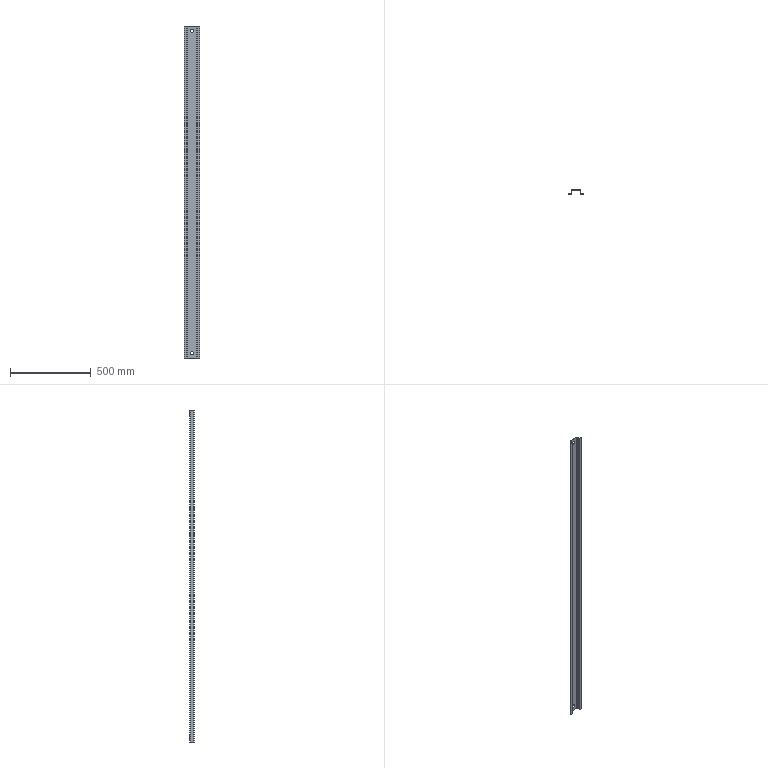Part | SolidWorks | features Cut 1, EdgeFlange 1, FlatPattern 1, ICE 1, SMBaseFlange 1, SheetMetal 1 | 1 solid | 42 faces | box 98.4 x 25 x 2051 mm | volume 236423 mm3 | plane 30 | cylinder 12 | commonest cylinder face diameters 2 x4 3.6 x4 20 x4
STEP:
#1=CARTESIAN_POINT('',(10.,-0.8,-995.5));
#2=VERTEX_POINT('',#1);
#3=CARTESIAN_POINT('',(-10.,-0.8,-995.5));
#4=VERTEX_POINT('',#3);
#5=CARTESIAN_POINT('',(0.,-0.8,-995.5));
#6=DIRECTION('',(0.,1.,0.));
#7=DIRECTION('',(-1.,0.,0.));
#8=AXIS2_PLACEMENT_3D('',#5,#6,#7);
#9=CIRCLE('',#8,10.);
#10=EDGE_CURVE('',#2,#4,#9,.T.);
#11=ORIENTED_EDGE('',*,*,#10,.F.);
#12=CARTESIAN_POINT('',(10.,0.,-995.5));
#13=VERTEX_POINT('',#12);
#14=CARTESIAN_POINT('',(10.,-10.,-995.5));
#15=DIRECTION('',(0.,1.,0.));
#16=VECTOR('',#15,1000.);
#17=LINE('',#14,#16);
#18=EDGE_CURVE('',#2,#13,#17,.T.);
#19=ORIENTED_EDGE('',*,*,#18,.T.);
#20=CARTESIAN_POINT('',(-10.,0.,-995.5));
#21=VERTEX_POINT('',#20);
#22=CARTESIAN_POINT('',(0.,0.,-995.5));
#23=DIRECTION('',(0.,1.,0.));
#24=DIRECTION('',(-1.,0.,0.));
#25=AXIS2_PLACEMENT_3D('',#22,#23,#24);
#26=CIRCLE('',#25,10.);
#27=EDGE_CURVE('',#13,#21,#26,.T.);
#28=ORIENTED_EDGE('',*,*,#27,.T.);
#29=CARTESIAN_POINT('',(-10.,-10.,-995.5));
#30=DIRECTION('',(0.,1.,0.));
#31=VECTOR('',#30,1000.);
#32=LINE('',#29,#31);
#33=EDGE_CURVE('',#4,#21,#32,.T.);
#34=ORIENTED_EDGE('',*,*,#33,.F.);
#35=EDGE_LOOP('',(#11,#19,#28,#34));
#36=FACE_OUTER_BOUND('',#35,.T.);
#37=CARTESIAN_POINT('',(0.,-10.,-995.5));
#38=DIRECTION('',(0.,1.,0.));
#39=DIRECTION('',(-1.,0.,0.));
#40=AXIS2_PLACEMENT_3D('',#37,#38,#39);
#41=CYLINDRICAL_SURFACE('',#40,10.);
#42=ADVANCED_FACE('',(#36),#41,.F.);
#43=CARTESIAN_POINT('',(10.,-0.8,995.5));
#44=VERTEX_POINT('',#43);
#45=CARTESIAN_POINT('',(-10.,-0.8,995.5));
#46=VERTEX_POINT('',#45);
#47=CARTESIAN_POINT('',(0.,-0.8,995.5));
#48=DIRECTION('',(0.,1.,0.));
#49=DIRECTION('',(-1.,0.,0.));
#50=AXIS2_PLACEMENT_3D('',#47,#48,#49);
#51=CIRCLE('',#50,10.);
#52=EDGE_CURVE('',#44,#46,#51,.T.);
#53=ORIENTED_EDGE('',*,*,#52,.F.);
#54=CARTESIAN_POINT('',(10.,0.,995.5));
#55=VERTEX_POINT('',#54);
#56=CARTESIAN_POINT('',(10.,-10.,995.5));
#57=DIRECTION('',(0.,1.,0.));
#58=VECTOR('',#57,1000.);
#59=LINE('',#56,#58);
#60=EDGE_CURVE('',#44,#55,#59,.T.);
#61=ORIENTED_EDGE('',*,*,#60,.T.);
#62=CARTESIAN_POINT('',(-10.,0.,995.5));
#63=VERTEX_POINT('',#62);
#64=CARTESIAN_POINT('',(0.,0.,995.5));
#65=DIRECTION('',(0.,1.,0.));
#66=DIRECTION('',(1.,0.,0.));
#67=AXIS2_PLACEMENT_3D('',#64,#65,#66);
#68=CIRCLE('',#67,10.);
#69=EDGE_CURVE('',#55,#63,#68,.T.);
#70=ORIENTED_EDGE('',*,*,#69,.T.);
#71=CARTESIAN_POINT('',(-10.,-10.,995.5));
#72=DIRECTION('',(0.,1.,0.));
#73=VECTOR('',#72,1000.);
#74=LINE('',#71,#73);
#75=EDGE_CURVE('',#46,#63,#74,.T.);
#76=ORIENTED_EDGE('',*,*,#75,.F.);
#77=EDGE_LOOP('',(#53,#61,#70,#76));
#78=FACE_OUTER_BOUND('',#77,.T.);
#79=CARTESIAN_POINT('',(0.,-10.,995.5));
#80=DIRECTION('',(0.,1.,0.));
#81=DIRECTION('',(-1.,0.,0.));
#82=AXIS2_PLACEMENT_3D('',#79,#80,#81);
#83=CYLINDRICAL_SURFACE('',#82,10.);
#84=ADVANCED_FACE('',(#78),#83,.F.);
#85=CARTESIAN_POINT('',(29.2,-23.2,-1025.5));
#86=VERTEX_POINT('',#85);
#87=CARTESIAN_POINT('',(29.2,-23.2,1025.5));
#88=VERTEX_POINT('',#87);
#89=CARTESIAN_POINT('',(29.2,-23.2,-1025.5));
#90=DIRECTION('',(0.,0.,1.));
#91=VECTOR('',#90,1000.);
#92=LINE('',#89,#91);
#93=EDGE_CURVE('',#86,#88,#92,.T.);
#94=ORIENTED_EDGE('',*,*,#93,.T.);
#95=CARTESIAN_POINT('',(29.2,-1.8,1025.5));
#96=VERTEX_POINT('',#95);
#97=CARTESIAN_POINT('',(29.2,0.,1025.5));
#98=DIRECTION('',(0.,-1.,0.));
#99=VECTOR('',#98,1000.);
#100=LINE('',#97,#99);
#101=EDGE_CURVE('',#96,#88,#100,.T.);
#102=ORIENTED_EDGE('',*,*,#101,.F.);
#103=CARTESIAN_POINT('',(29.2,-1.8,-1025.5));
#104=VERTEX_POINT('',#103);
#105=CARTESIAN_POINT('',(29.2,-1.8,1025.5));
#106=DIRECTION('',(0.,0.,-1.));
#107=VECTOR('',#106,1000.);
#108=LINE('',#105,#107);
#109=EDGE_CURVE('',#96,#104,#108,.T.);
#110=ORIENTED_EDGE('',*,*,#109,.T.);
#111=CARTESIAN_POINT('',(29.2,0.,-1025.5));
#112=DIRECTION('',(0.,-1.,0.));
#113=VECTOR('',#112,1000.);
#114=LINE('',#111,#113);
#115=EDGE_CURVE('',#104,#86,#114,.T.);
#116=ORIENTED_EDGE('',*,*,#115,.T.);
#117=EDGE_LOOP('',(#94,#102,#110,#116));
#118=FACE_OUTER_BOUND('',#117,.T.);
#119=CARTESIAN_POINT('',(29.2,0.,1025.5));
#120=DIRECTION('',(1.,0.,0.));
#121=DIRECTION('',(0.,1.,0.));
#122=AXIS2_PLACEMENT_3D('',#119,#120,#121);
#123=PLANE('',#122);
#124=ADVANCED_FACE('',(#118),#123,.F.);
#125=CARTESIAN_POINT('',(30.,-1.8,1025.5));
#126=VERTEX_POINT('',#125);
#127=CARTESIAN_POINT('',(30.,-23.2,1025.5));
#128=VERTEX_POINT('',#127);
#129=CARTESIAN_POINT('',(30.,0.,1025.5));
#130=DIRECTION('',(0.,-1.,0.));
#131=VECTOR('',#130,1000.);
#132=LINE('',#129,#131);
#133=EDGE_CURVE('',#126,#128,#132,.T.);
#134=ORIENTED_EDGE('',*,*,#133,.T.);
#135=CARTESIAN_POINT('',(30.,-23.2,-1025.5));
#136=VERTEX_POINT('',#135);
#137=CARTESIAN_POINT('',(30.,-23.2,-1025.5));
#138=DIRECTION('',(0.,0.,1.));
#139=VECTOR('',#138,1000.);
#140=LINE('',#137,#139);
#141=EDGE_CURVE('',#136,#128,#140,.T.);
#142=ORIENTED_EDGE('',*,*,#141,.F.);
#143=CARTESIAN_POINT('',(30.,-1.8,-1025.5));
#144=VERTEX_POINT('',#143);
#145=CARTESIAN_POINT('',(30.,0.,-1025.5));
#146=DIRECTION('',(0.,-1.,0.));
#147=VECTOR('',#146,1000.);
#148=LINE('',#145,#147);
#149=EDGE_CURVE('',#144,#136,#148,.T.);
#150=ORIENTED_EDGE('',*,*,#149,.F.);
#151=CARTESIAN_POINT('',(30.,-1.8,1025.5));
#152=DIRECTION('',(0.,0.,-1.));
#153=VECTOR('',#152,1000.);
#154=LINE('',#151,#153);
#155=EDGE_CURVE('',#126,#144,#154,.T.);
#156=ORIENTED_EDGE('',*,*,#155,.F.);
#157=EDGE_LOOP('',(#134,#142,#150,#156));
#158=FACE_OUTER_BOUND('',#157,.T.);
#159=CARTESIAN_POINT('',(30.,0.,1025.5));
#160=DIRECTION('',(1.,0.,0.));
#161=DIRECTION('',(0.,1.,0.));
#162=AXIS2_PLACEMENT_3D('',#159,#160,#161);
#163=PLANE('',#162);
#164=ADVANCED_FACE('',(#158),#163,.T.);
#165=CARTESIAN_POINT('',(30.,-23.2,-1025.5));
#166=DIRECTION('',(-1.,0.,0.));
#167=VECTOR('',#166,1000.);
#168=LINE('',#165,#167);
#169=EDGE_CURVE('',#136,#86,#168,.T.);
#170=ORIENTED_EDGE('',*,*,#169,.T.);
#171=ORIENTED_EDGE('',*,*,#115,.F.);
#172=CARTESIAN_POINT('',(29.2,-1.8,-1025.5));
#173=DIRECTION('',(1.,0.,0.));
#174=VECTOR('',#173,1000.);
#175=LINE('',#172,#174);
#176=EDGE_CURVE('',#104,#144,#175,.T.);
#177=ORIENTED_EDGE('',*,*,#176,.T.);
#178=ORIENTED_EDGE('',*,*,#149,.T.);
#179=EDGE_LOOP('',(#170,#171,#177,#178));
#180=FACE_OUTER_BOUND('',#179,.T.);
#181=CARTESIAN_POINT('',(28.2,-1.8,-1025.5));
#182=DIRECTION('',(0.,0.,1.));
#183=DIRECTION('',(1.,0.,0.));
#184=AXIS2_PLACEMENT_3D('',#181,#182,#183);
#185=PLANE('',#184);
#186=ADVANCED_FACE('',(#180),#185,.F.);
#187=CARTESIAN_POINT('',(-30.,-23.2,-1025.5));
#188=VERTEX_POINT('',#187);
#189=CARTESIAN_POINT('',(-30.,-1.8,-1025.5));
#190=VERTEX_POINT('',#189);
#191=CARTESIAN_POINT('',(-30.,-25.,-1025.5));
#192=DIRECTION('',(0.,1.,0.));
#193=VECTOR('',#192,1000.);
#194=LINE('',#191,#193);
#195=EDGE_CURVE('',#188,#190,#194,.T.);
#196=ORIENTED_EDGE('',*,*,#195,.F.);
#197=CARTESIAN_POINT('',(-30.,-23.2,1025.5));
#198=VERTEX_POINT('',#197);
#199=CARTESIAN_POINT('',(-30.,-23.2,1025.5));
#200=DIRECTION('',(0.,0.,-1.));
#201=VECTOR('',#200,1000.);
#202=LINE('',#199,#201);
#203=EDGE_CURVE('',#198,#188,#202,.T.);
#204=ORIENTED_EDGE('',*,*,#203,.F.);
#205=CARTESIAN_POINT('',(-30.,-1.8,1025.5));
#206=VERTEX_POINT('',#205);
#207=CARTESIAN_POINT('',(-30.,-25.,1025.5));
#208=DIRECTION('',(0.,1.,0.));
#209=VECTOR('',#208,1000.);
#210=LINE('',#207,#209);
#211=EDGE_CURVE('',#198,#206,#210,.T.);
#212=ORIENTED_EDGE('',*,*,#211,.T.);
#213=CARTESIAN_POINT('',(-30.,-1.8,1025.5));
#214=DIRECTION('',(0.,0.,-1.));
#215=VECTOR('',#214,1000.);
#216=LINE('',#213,#215);
#217=EDGE_CURVE('',#206,#190,#216,.T.);
#218=ORIENTED_EDGE('',*,*,#217,.T.);
#219=EDGE_LOOP('',(#196,#204,#212,#218));
#220=FACE_OUTER_BOUND('',#219,.T.);
#221=CARTESIAN_POINT('',(-30.,-25.,1025.5));
#222=DIRECTION('',(-1.,0.,0.));
#223=DIRECTION('',(0.,0.,1.));
#224=AXIS2_PLACEMENT_3D('',#221,#222,#223);
#225=PLANE('',#224);
#226=ADVANCED_FACE('',(#220),#225,.T.);
#227=CARTESIAN_POINT('',(-29.2,-23.2,1025.5));
#228=VERTEX_POINT('',#227);
#229=CARTESIAN_POINT('',(-29.2,-23.2,-1025.5));
#230=VERTEX_POINT('',#229);
#231=CARTESIAN_POINT('',(-29.2,-23.2,1025.5));
#232=DIRECTION('',(0.,0.,-1.));
#233=VECTOR('',#232,1000.);
#234=LINE('',#231,#233);
#235=EDGE_CURVE('',#228,#230,#234,.T.);
#236=ORIENTED_EDGE('',*,*,#235,.T.);
#237=CARTESIAN_POINT('',(-29.2,-1.8,-1025.5));
#238=VERTEX_POINT('',#237);
#239=CARTESIAN_POINT('',(-29.2,-25.,-1025.5));
#240=DIRECTION('',(0.,1.,0.));
#241=VECTOR('',#240,1000.);
#242=LINE('',#239,#241);
#243=EDGE_CURVE('',#230,#238,#242,.T.);
#244=ORIENTED_EDGE('',*,*,#243,.T.);
#245=CARTESIAN_POINT('',(-29.2,-1.8,1025.5));
#246=VERTEX_POINT('',#245);
#247=CARTESIAN_POINT('',(-29.2,-1.8,1025.5));
#248=DIRECTION('',(0.,0.,-1.));
#249=VECTOR('',#248,1000.);
#250=LINE('',#247,#249);
#251=EDGE_CURVE('',#246,#238,#250,.T.);
#252=ORIENTED_EDGE('',*,*,#251,.F.);
#253=CARTESIAN_POINT('',(-29.2,-25.,1025.5));
#254=DIRECTION('',(0.,1.,0.));
#255=VECTOR('',#254,1000.);
#256=LINE('',#253,#255);
#257=EDGE_CURVE('',#228,#246,#256,.T.);
#258=ORIENTED_EDGE('',*,*,#257,.F.);
#259=EDGE_LOOP('',(#236,#244,#252,#258));
#260=FACE_OUTER_BOUND('',#259,.T.);
#261=CARTESIAN_POINT('',(-29.2,-25.,1025.5));
#262=DIRECTION('',(-1.,0.,0.));
#263=DIRECTION('',(0.,0.,1.));
#264=AXIS2_PLACEMENT_3D('',#261,#262,#263);
#265=PLANE('',#264);
#266=ADVANCED_FACE('',(#260),#265,.F.);
#267=ORIENTED_EDGE('',*,*,#211,.F.);
#268=CARTESIAN_POINT('',(-30.,-23.2,1025.5));
#269=DIRECTION('',(1.,0.,0.));
#270=VECTOR('',#269,1000.);
#271=LINE('',#268,#270);
#272=EDGE_CURVE('',#198,#228,#271,.T.);
#273=ORIENTED_EDGE('',*,*,#272,.T.);
#274=ORIENTED_EDGE('',*,*,#257,.T.);
#275=CARTESIAN_POINT('',(-29.2,-1.8,1025.5));
#276=DIRECTION('',(-1.,0.,0.));
#277=VECTOR('',#276,1000.);
#278=LINE('',#275,#277);
#279=EDGE_CURVE('',#246,#206,#278,.T.);
#280=ORIENTED_EDGE('',*,*,#279,.T.);
#281=EDGE_LOOP('',(#267,#273,#274,#280));
#282=FACE_OUTER_BOUND('',#281,.T.);
#283=CARTESIAN_POINT('',(28.2,-1.8,1025.5));
#284=DIRECTION('',(0.,0.,1.));
#285=DIRECTION('',(1.,0.,0.));
#286=AXIS2_PLACEMENT_3D('',#283,#284,#285);
#287=PLANE('',#286);
#288=ADVANCED_FACE('',(#282),#287,.T.);
#289=CARTESIAN_POINT('',(-28.2,0.,1025.5));
#290=VERTEX_POINT('',#289);
#291=CARTESIAN_POINT('',(-28.2,-0.8,1025.5));
#292=VERTEX_POINT('',#291);
#293=CARTESIAN_POINT('',(-28.2,0.,1025.5));
#294=DIRECTION('',(0.,-1.,0.));
#295=VECTOR('',#294,1000.);
#296=LINE('',#293,#295);
#297=EDGE_CURVE('',#290,#292,#296,.T.);
#298=ORIENTED_EDGE('',*,*,#297,.F.);
#299=CARTESIAN_POINT('',(-28.2,-1.8,1025.5));
#300=DIRECTION('',(0.,0.,-1.));
#301=DIRECTION('',(1.,0.,0.));
#302=AXIS2_PLACEMENT_3D('',#299,#300,#301);
#303=CIRCLE('',#302,1.8);
#304=EDGE_CURVE('',#206,#290,#303,.T.);
#305=ORIENTED_EDGE('',*,*,#304,.F.);
#306=ORIENTED_EDGE('',*,*,#279,.F.);
#307=CARTESIAN_POINT('',(-28.2,-1.8,1025.5));
#308=DIRECTION('',(0.,0.,-1.));
#309=DIRECTION('',(1.,0.,0.));
#310=AXIS2_PLACEMENT_3D('',#307,#308,#309);
#311=CIRCLE('',#310,1.);
#312=EDGE_CURVE('',#246,#292,#311,.T.);
#313=ORIENTED_EDGE('',*,*,#312,.T.);
#314=EDGE_LOOP('',(#298,#305,#306,#313));
#315=FACE_OUTER_BOUND('',#314,.T.);
#316=CARTESIAN_POINT('',(-28.2,0.,1025.5));
#317=DIRECTION('',(0.,0.,1.));
#318=DIRECTION('',(1.,0.,0.));
#319=AXIS2_PLACEMENT_3D('',#316,#317,#318);
#320=PLANE('',#319);
#321=ADVANCED_FACE('',(#315),#320,.T.);
#322=CARTESIAN_POINT('',(28.2,0.,1025.5));
#323=VERTEX_POINT('',#322);
#324=CARTESIAN_POINT('',(-30.,0.,1025.5));
#325=DIRECTION('',(1.,0.,0.));
#326=VECTOR('',#325,1000.);
#327=LINE('',#324,#326);
#328=EDGE_CURVE('',#290,#323,#327,.T.);
#329=ORIENTED_EDGE('',*,*,#328,.F.);
#330=ORIENTED_EDGE('',*,*,#297,.T.);
#331=CARTESIAN_POINT('',(28.2,-0.8,1025.5));
#332=VERTEX_POINT('',#331);
#333=CARTESIAN_POINT('',(-30.,-0.8,1025.5));
#334=DIRECTION('',(1.,0.,0.));
#335=VECTOR('',#334,1000.);
#336=LINE('',#333,#335);
#337=EDGE_CURVE('',#292,#332,#336,.T.);
#338=ORIENTED_EDGE('',*,*,#337,.T.);
#339=CARTESIAN_POINT('',(28.2,-0.8,1025.5));
#340=DIRECTION('',(0.,1.,0.));
#341=VECTOR('',#340,1000.);
#342=LINE('',#339,#341);
#343=EDGE_CURVE('',#332,#323,#342,.T.);
#344=ORIENTED_EDGE('',*,*,#343,.T.);
#345=EDGE_LOOP('',(#329,#330,#338,#344));
#346=FACE_OUTER_BOUND('',#345,.T.);
#347=CARTESIAN_POINT('',(-29.2,-1.8,1025.5));
#348=DIRECTION('',(0.,0.,1.));
#349=DIRECTION('',(1.,0.,0.));
#350=AXIS2_PLACEMENT_3D('',#347,#348,#349);
#351=PLANE('',#350);
#352=ADVANCED_FACE('',(#346),#351,.T.);
#353=CARTESIAN_POINT('',(-30.,-1.8,-1025.5));
#354=DIRECTION('',(1.,0.,0.));
#355=VECTOR('',#354,1000.);
#356=LINE('',#353,#355);
#357=EDGE_CURVE('',#190,#238,#356,.T.);
#358=ORIENTED_EDGE('',*,*,#357,.F.);
#359=CARTESIAN_POINT('',(-28.2,0.,-1025.5));
#360=VERTEX_POINT('',#359);
#361=CARTESIAN_POINT('',(-28.2,-1.8,-1025.5));
#362=DIRECTION('',(0.,0.,-1.));
#363=DIRECTION('',(1.,0.,0.));
#364=AXIS2_PLACEMENT_3D('',#361,#362,#363);
#365=CIRCLE('',#364,1.8);
#366=EDGE_CURVE('',#190,#360,#365,.T.);
#367=ORIENTED_EDGE('',*,*,#366,.T.);
#368=CARTESIAN_POINT('',(-28.2,-0.8,-1025.5));
#369=VERTEX_POINT('',#368);
#370=CARTESIAN_POINT('',(-28.2,-0.8,-1025.5));
#371=DIRECTION('',(0.,1.,0.));
#372=VECTOR('',#371,1000.);
#373=LINE('',#370,#372);
#374=EDGE_CURVE('',#369,#360,#373,.T.);
#375=ORIENTED_EDGE('',*,*,#374,.F.);
#376=CARTESIAN_POINT('',(-28.2,-1.8,-1025.5));
#377=DIRECTION('',(0.,0.,-1.));
#378=DIRECTION('',(1.,0.,0.));
#379=AXIS2_PLACEMENT_3D('',#376,#377,#378);
#380=CIRCLE('',#379,1.);
#381=EDGE_CURVE('',#238,#369,#380,.T.);
#382=ORIENTED_EDGE('',*,*,#381,.F.);
#383=EDGE_LOOP('',(#358,#367,#375,#382));
#384=FACE_OUTER_BOUND('',#383,.T.);
#385=CARTESIAN_POINT('',(-30.,-1.8,-1025.5));
#386=DIRECTION('',(0.,0.,-1.));
#387=DIRECTION('',(-1.,0.,0.));
#388=AXIS2_PLACEMENT_3D('',#385,#386,#387);
#389=PLANE('',#388);
#390=ADVANCED_FACE('',(#384),#389,.T.);
#391=CARTESIAN_POINT('',(-30.,-23.2,-1025.5));
#392=DIRECTION('',(1.,0.,0.));
#393=VECTOR('',#392,1000.);
#394=LINE('',#391,#393);
#395=EDGE_CURVE('',#188,#230,#394,.T.);
#396=ORIENTED_EDGE('',*,*,#395,.F.);
#397=ORIENTED_EDGE('',*,*,#195,.T.);
#398=ORIENTED_EDGE('',*,*,#357,.T.);
#399=ORIENTED_EDGE('',*,*,#243,.F.);
#400=EDGE_LOOP('',(#396,#397,#398,#399));
#401=FACE_OUTER_BOUND('',#400,.T.);
#402=CARTESIAN_POINT('',(-28.2,-0.8,-1025.5));
#403=DIRECTION('',(0.,0.,-1.));
#404=DIRECTION('',(-1.,0.,0.));
#405=AXIS2_PLACEMENT_3D('',#402,#403,#404);
#406=PLANE('',#405);
#407=ADVANCED_FACE('',(#401),#406,.T.);
#408=CARTESIAN_POINT('',(30.,-1.8,1025.5));
#409=DIRECTION('',(-1.,0.,0.));
#410=VECTOR('',#409,1000.);
#411=LINE('',#408,#410);
#412=EDGE_CURVE('',#126,#96,#411,.T.);
#413=ORIENTED_EDGE('',*,*,#412,.F.);
#414=CARTESIAN_POINT('',(28.2,-1.8,1025.5));
#415=DIRECTION('',(0.,0.,-1.));
#416=DIRECTION('',(1.,0.,0.));
#417=AXIS2_PLACEMENT_3D('',#414,#415,#416);
#418=CIRCLE('',#417,1.8);
#419=EDGE_CURVE('',#323,#126,#418,.T.);
#420=ORIENTED_EDGE('',*,*,#419,.F.);
#421=ORIENTED_EDGE('',*,*,#343,.F.);
#422=CARTESIAN_POINT('',(28.2,-1.8,1025.5));
#423=DIRECTION('',(0.,0.,-1.));
#424=DIRECTION('',(1.,0.,0.));
#425=AXIS2_PLACEMENT_3D('',#422,#423,#424);
#426=CIRCLE('',#425,1.);
#427=EDGE_CURVE('',#332,#96,#426,.T.);
#428=ORIENTED_EDGE('',*,*,#427,.T.);
#429=EDGE_LOOP('',(#413,#420,#421,#428));
#430=FACE_OUTER_BOUND('',#429,.T.);
#431=CARTESIAN_POINT('',(30.,-1.8,1025.5));
#432=DIRECTION('',(0.,0.,1.));
#433=DIRECTION('',(1.,0.,0.));
#434=AXIS2_PLACEMENT_3D('',#431,#432,#433);
#435=PLANE('',#434);
#436=ADVANCED_FACE('',(#430),#435,.T.);
#437=CARTESIAN_POINT('',(30.,-23.2,1025.5));
#438=DIRECTION('',(-1.,0.,0.));
#439=VECTOR('',#438,1000.);
#440=LINE('',#437,#439);
#441=EDGE_CURVE('',#128,#88,#440,.T.);
#442=ORIENTED_EDGE('',*,*,#441,.F.);
#443=ORIENTED_EDGE('',*,*,#133,.F.);
#444=ORIENTED_EDGE('',*,*,#412,.T.);
#445=ORIENTED_EDGE('',*,*,#101,.T.);
#446=EDGE_LOOP('',(#442,#443,#444,#445));
#447=FACE_OUTER_BOUND('',#446,.T.);
#448=CARTESIAN_POINT('',(28.2,-0.8,1025.5));
#449=DIRECTION('',(0.,0.,1.));
#450=DIRECTION('',(1.,0.,0.));
#451=AXIS2_PLACEMENT_3D('',#448,#449,#450);
#452=PLANE('',#451);
#453=ADVANCED_FACE('',(#447),#452,.T.);
#454=CARTESIAN_POINT('',(28.2,0.,-1025.5));
#455=VERTEX_POINT('',#454);
#456=CARTESIAN_POINT('',(28.2,-0.8,-1025.5));
#457=VERTEX_POINT('',#456);
#458=CARTESIAN_POINT('',(28.2,0.,-1025.5));
#459=DIRECTION('',(0.,-1.,0.));
#460=VECTOR('',#459,1000.);
#461=LINE('',#458,#460);
#462=EDGE_CURVE('',#455,#457,#461,.T.);
#463=ORIENTED_EDGE('',*,*,#462,.F.);
#464=CARTESIAN_POINT('',(28.2,-1.8,-1025.5));
#465=DIRECTION('',(0.,0.,-1.));
#466=DIRECTION('',(1.,0.,0.));
#467=AXIS2_PLACEMENT_3D('',#464,#465,#466);
#468=CIRCLE('',#467,1.8);
#469=EDGE_CURVE('',#455,#144,#468,.T.);
#470=ORIENTED_EDGE('',*,*,#469,.T.);
#471=ORIENTED_EDGE('',*,*,#176,.F.);
#472=CARTESIAN_POINT('',(28.2,-1.8,-1025.5));
#473=DIRECTION('',(0.,0.,-1.));
#474=DIRECTION('',(1.,0.,0.));
#475=AXIS2_PLACEMENT_3D('',#472,#473,#474);
#476=CIRCLE('',#475,1.);
#477=EDGE_CURVE('',#457,#104,#476,.T.);
#478=ORIENTED_EDGE('',*,*,#477,.F.);
#479=EDGE_LOOP('',(#463,#470,#471,#478));
#480=FACE_OUTER_BOUND('',#479,.T.);
#481=CARTESIAN_POINT('',(28.2,0.,-1025.5));
#482=DIRECTION('',(0.,0.,-1.));
#483=DIRECTION('',(-1.,0.,0.));
#484=AXIS2_PLACEMENT_3D('',#481,#482,#483);
#485=PLANE('',#484);
#486=ADVANCED_FACE('',(#480),#485,.T.);
#487=CARTESIAN_POINT('',(-30.,0.,-1025.5));
#488=DIRECTION('',(1.,0.,0.));
#489=VECTOR('',#488,1000.);
#490=LINE('',#487,#489);
#491=EDGE_CURVE('',#360,#455,#490,.T.);
#492=ORIENTED_EDGE('',*,*,#491,.T.);
#493=ORIENTED_EDGE('',*,*,#462,.T.);
#494=CARTESIAN_POINT('',(-30.,-0.8,-1025.5));
#495=DIRECTION('',(1.,0.,0.));
#496=VECTOR('',#495,1000.);
#497=LINE('',#494,#496);
#498=EDGE_CURVE('',#369,#457,#497,.T.);
#499=ORIENTED_EDGE('',*,*,#498,.F.);
#500=ORIENTED_EDGE('',*,*,#374,.T.);
#501=EDGE_LOOP('',(#492,#493,#499,#500));
#502=FACE_OUTER_BOUND('',#501,.T.);
#503=CARTESIAN_POINT('',(29.2,-1.8,-1025.5));
#504=DIRECTION('',(0.,0.,-1.));
#505=DIRECTION('',(-1.,0.,0.));
#506=AXIS2_PLACEMENT_3D('',#503,#504,#505);
#507=PLANE('',#506);
#508=ADVANCED_FACE('',(#502),#507,.T.);
#509=ORIENTED_EDGE('',*,*,#469,.F.);
#510=CARTESIAN_POINT('',(28.2,0.,1025.5));
#511=DIRECTION('',(0.,0.,-1.));
#512=VECTOR('',#511,1000.);
#513=LINE('',#510,#512);
#514=EDGE_CURVE('',#323,#455,#513,.T.);
#515=ORIENTED_EDGE('',*,*,#514,.F.);
#516=ORIENTED_EDGE('',*,*,#419,.T.);
#517=ORIENTED_EDGE('',*,*,#155,.T.);
#518=EDGE_LOOP('',(#509,#515,#516,#517));
#519=FACE_OUTER_BOUND('',#518,.T.);
#520=CARTESIAN_POINT('',(28.2,-1.8,1025.5));
#521=DIRECTION('',(0.,0.,-1.));
#522=DIRECTION('',(-1.,0.,0.));
#523=AXIS2_PLACEMENT_3D('',#520,#521,#522);
#524=CYLINDRICAL_SURFACE('',#523,1.8);
#525=ADVANCED_FACE('',(#519),#524,.T.);
#526=CARTESIAN_POINT('',(0.,0.,-995.5));
#527=DIRECTION('',(0.,1.,0.));
#528=DIRECTION('',(-1.,0.,0.));
#529=AXIS2_PLACEMENT_3D('',#526,#527,#528);
#530=CIRCLE('',#529,10.);
#531=EDGE_CURVE('',#21,#13,#530,.T.);
#532=ORIENTED_EDGE('',*,*,#531,.F.);
#533=ORIENTED_EDGE('',*,*,#27,.F.);
#534=EDGE_LOOP('',(#532,#533));
#535=FACE_BOUND('',#534,.T.);
#536=CARTESIAN_POINT('',(0.,0.,995.5));
#537=DIRECTION('',(0.,1.,0.));
#538=DIRECTION('',(1.,0.,0.));
#539=AXIS2_PLACEMENT_3D('',#536,#537,#538);
#540=CIRCLE('',#539,10.);
#541=EDGE_CURVE('',#63,#55,#540,.T.);
#542=ORIENTED_EDGE('',*,*,#541,.F.);
#543=ORIENTED_EDGE('',*,*,#69,.F.);
#544=EDGE_LOOP('',(#542,#543));
#545=FACE_BOUND('',#544,.T.);
#546=ORIENTED_EDGE('',*,*,#491,.F.);
#547=CARTESIAN_POINT('',(-28.2,0.,1025.5));
#548=DIRECTION('',(0.,0.,-1.));
#549=VECTOR('',#548,1000.);
#550=LINE('',#547,#549);
#551=EDGE_CURVE('',#290,#360,#550,.T.);
#552=ORIENTED_EDGE('',*,*,#551,.F.);
#553=ORIENTED_EDGE('',*,*,#328,.T.);
#554=ORIENTED_EDGE('',*,*,#514,.T.);
#555=EDGE_LOOP('',(#546,#552,#553,#554));
#556=FACE_OUTER_BOUND('',#555,.T.);
#557=CARTESIAN_POINT('',(-30.,0.,1025.5));
#558=DIRECTION('',(0.,1.,0.));
#559=DIRECTION('',(-1.,0.,0.));
#560=AXIS2_PLACEMENT_3D('',#557,#558,#559);
#561=PLANE('',#560);
#562=ADVANCED_FACE('',(#535,#545,#556),#561,.T.);
#563=ORIENTED_EDGE('',*,*,#366,.F.);
#564=ORIENTED_EDGE('',*,*,#217,.F.);
#565=ORIENTED_EDGE('',*,*,#304,.T.);
#566=ORIENTED_EDGE('',*,*,#551,.T.);
#567=EDGE_LOOP('',(#563,#564,#565,#566));
#568=FACE_OUTER_BOUND('',#567,.T.);
#569=CARTESIAN_POINT('',(-28.2,-1.8,1025.5));
#570=DIRECTION('',(0.,0.,-1.));
#571=DIRECTION('',(-1.,0.,0.));
#572=AXIS2_PLACEMENT_3D('',#569,#570,#571);
#573=CYLINDRICAL_SURFACE('',#572,1.8);
#574=ADVANCED_FACE('',(#568),#573,.T.);
#575=ORIENTED_EDGE('',*,*,#381,.T.);
#576=CARTESIAN_POINT('',(-28.2,-0.8,1025.5));
#577=DIRECTION('',(0.,0.,-1.));
#578=VECTOR('',#577,1000.);
#579=LINE('',#576,#578);
#580=EDGE_CURVE('',#292,#369,#579,.T.);
#581=ORIENTED_EDGE('',*,*,#580,.F.);
#582=ORIENTED_EDGE('',*,*,#312,.F.);
#583=ORIENTED_EDGE('',*,*,#251,.T.);
#584=EDGE_LOOP('',(#575,#581,#582,#583));
#585=FACE_OUTER_BOUND('',#584,.T.);
#586=CARTESIAN_POINT('',(-28.2,-1.8,1025.5));
#587=DIRECTION('',(0.,0.,-1.));
#588=DIRECTION('',(-1.,0.,0.));
#589=AXIS2_PLACEMENT_3D('',#586,#587,#588);
#590=CYLINDRICAL_SURFACE('',#589,1.);
#591=ADVANCED_FACE('',(#585),#590,.F.);
#592=CARTESIAN_POINT('',(0.,-0.8,-995.5));
#593=DIRECTION('',(0.,1.,0.));
#594=DIRECTION('',(-1.,0.,0.));
#595=AXIS2_PLACEMENT_3D('',#592,#593,#594);
#596=CIRCLE('',#595,10.);
#597=EDGE_CURVE('',#4,#2,#596,.T.);
#598=ORIENTED_EDGE('',*,*,#597,.T.);
#599=ORIENTED_EDGE('',*,*,#10,.T.);
#600=EDGE_LOOP('',(#598,#599));
#601=FACE_BOUND('',#600,.T.);
#602=CARTESIAN_POINT('',(0.,-0.8,995.5));
#603=DIRECTION('',(0.,1.,0.));
#604=DIRECTION('',(-1.,0.,0.));
#605=AXIS2_PLACEMENT_3D('',#602,#603,#604);
#606=CIRCLE('',#605,10.);
#607=EDGE_CURVE('',#46,#44,#606,.T.);
#608=ORIENTED_EDGE('',*,*,#607,.T.);
#609=ORIENTED_EDGE('',*,*,#52,.T.);
#610=EDGE_LOOP('',(#608,#609));
#611=FACE_BOUND('',#610,.T.);
#612=ORIENTED_EDGE('',*,*,#498,.T.);
#613=CARTESIAN_POINT('',(28.2,-0.8,1025.5));
#614=DIRECTION('',(0.,0.,-1.));
#615=VECTOR('',#614,1000.);
#616=LINE('',#613,#615);
#617=EDGE_CURVE('',#332,#457,#616,.T.);
#618=ORIENTED_EDGE('',*,*,#617,.F.);
#619=ORIENTED_EDGE('',*,*,#337,.F.);
#620=ORIENTED_EDGE('',*,*,#580,.T.);
#621=EDGE_LOOP('',(#612,#618,#619,#620));
#622=FACE_OUTER_BOUND('',#621,.T.);
#623=CARTESIAN_POINT('',(-30.,-0.8,1025.5));
#624=DIRECTION('',(0.,1.,0.));
#625=DIRECTION('',(-1.,0.,0.));
#626=AXIS2_PLACEMENT_3D('',#623,#624,#625);
#627=PLANE('',#626);
#628=ADVANCED_FACE('',(#601,#611,#622),#627,.F.);
#629=ORIENTED_EDGE('',*,*,#477,.T.);
#630=ORIENTED_EDGE('',*,*,#109,.F.);
#631=ORIENTED_EDGE('',*,*,#427,.F.);
#632=ORIENTED_EDGE('',*,*,#617,.T.);
#633=EDGE_LOOP('',(#629,#630,#631,#632));
#634=FACE_OUTER_BOUND('',#633,.T.);
#635=CARTESIAN_POINT('',(28.2,-1.8,1025.5));
#636=DIRECTION('',(0.,0.,-1.));
#637=DIRECTION('',(-1.,0.,0.));
#638=AXIS2_PLACEMENT_3D('',#635,#636,#637);
#639=CYLINDRICAL_SURFACE('',#638,1.);
#640=ADVANCED_FACE('',(#634),#639,.F.);
#641=CARTESIAN_POINT('',(-31.,-24.2,-1025.5));
#642=VERTEX_POINT('',#641);
#643=CARTESIAN_POINT('',(-31.,-25.,-1025.5));
#644=VERTEX_POINT('',#643);
#645=CARTESIAN_POINT('',(-31.,-25.,-1025.5));
#646=DIRECTION('',(0.,-1.,0.));
#647=VECTOR('',#646,1000.);
#648=LINE('',#645,#647);
#649=EDGE_CURVE('',#642,#644,#648,.T.);
#650=ORIENTED_EDGE('',*,*,#649,.F.);
#651=CARTESIAN_POINT('',(-31.,-23.2,-1025.5));
#652=DIRECTION('',(0.,0.,-1.));
#653=DIRECTION('',(1.,0.,0.));
#654=AXIS2_PLACEMENT_3D('',#651,#652,#653);
#655=CIRCLE('',#654,1.);
#656=EDGE_CURVE('',#188,#642,#655,.T.);
#657=ORIENTED_EDGE('',*,*,#656,.F.);
#658=ORIENTED_EDGE('',*,*,#395,.T.);
#659=CARTESIAN_POINT('',(-31.,-23.2,-1025.5));
#660=DIRECTION('',(0.,0.,-1.));
#661=DIRECTION('',(1.,0.,0.));
#662=AXIS2_PLACEMENT_3D('',#659,#660,#661);
#663=CIRCLE('',#662,1.8);
#664=EDGE_CURVE('',#230,#644,#663,.T.);
#665=ORIENTED_EDGE('',*,*,#664,.T.);
#666=EDGE_LOOP('',(#650,#657,#658,#665));
#667=FACE_OUTER_BOUND('',#666,.T.);
#668=CARTESIAN_POINT('',(-31.,-23.2,-1025.5));
#669=DIRECTION('',(0.,0.,-1.));
#670=DIRECTION('',(-1.,0.,0.));
#671=AXIS2_PLACEMENT_3D('',#668,#669,#670);
#672=PLANE('',#671);
#673=ADVANCED_FACE('',(#667),#672,.T.);
#674=CARTESIAN_POINT('',(-31.,-24.2,1025.5));
#675=VERTEX_POINT('',#674);
#676=CARTESIAN_POINT('',(-31.,-23.2,1025.5));
#677=DIRECTION('',(0.,0.,1.));
#678=DIRECTION('',(1.,0.,0.));
#679=AXIS2_PLACEMENT_3D('',#676,#677,#678);
#680=CIRCLE('',#679,1.);
#681=EDGE_CURVE('',#675,#198,#680,.T.);
#682=ORIENTED_EDGE('',*,*,#681,.F.);
#683=CARTESIAN_POINT('',(-31.,-25.,1025.5));
#684=VERTEX_POINT('',#683);
#685=CARTESIAN_POINT('',(-31.,-24.2,1025.5));
#686=DIRECTION('',(0.,-1.,0.));
#687=VECTOR('',#686,1000.);
#688=LINE('',#685,#687);
#689=EDGE_CURVE('',#675,#684,#688,.T.);
#690=ORIENTED_EDGE('',*,*,#689,.T.);
#691=CARTESIAN_POINT('',(-31.,-23.2,1025.5));
#692=DIRECTION('',(0.,0.,1.));
#693=DIRECTION('',(1.,0.,0.));
#694=AXIS2_PLACEMENT_3D('',#691,#692,#693);
#695=CIRCLE('',#694,1.8);
#696=EDGE_CURVE('',#684,#228,#695,.T.);
#697=ORIENTED_EDGE('',*,*,#696,.T.);
#698=ORIENTED_EDGE('',*,*,#272,.F.);
#699=EDGE_LOOP('',(#682,#690,#697,#698));
#700=FACE_OUTER_BOUND('',#699,.T.);
#701=CARTESIAN_POINT('',(-31.,-23.2,1025.5));
#702=DIRECTION('',(0.,0.,-1.));
#703=DIRECTION('',(-1.,0.,0.));
#704=AXIS2_PLACEMENT_3D('',#701,#702,#703);
#705=PLANE('',#704);
#706=ADVANCED_FACE('',(#700),#705,.F.);
#707=ORIENTED_EDGE('',*,*,#235,.F.);
#708=ORIENTED_EDGE('',*,*,#696,.F.);
#709=CARTESIAN_POINT('',(-31.,-25.,-1025.5));
#710=DIRECTION('',(0.,0.,-1.));
#711=VECTOR('',#710,1000.);
#712=LINE('',#709,#711);
#713=EDGE_CURVE('',#684,#644,#712,.T.);
#714=ORIENTED_EDGE('',*,*,#713,.T.);
#715=ORIENTED_EDGE('',*,*,#664,.F.);
#716=EDGE_LOOP('',(#707,#708,#714,#715));
#717=FACE_OUTER_BOUND('',#716,.T.);
#718=CARTESIAN_POINT('',(-31.,-23.2,1025.5));
#719=DIRECTION('',(0.,0.,1.));
#720=DIRECTION('',(0.,-1.,0.));
#721=AXIS2_PLACEMENT_3D('',#718,#719,#720);
#722=CYLINDRICAL_SURFACE('',#721,1.8);
#723=ADVANCED_FACE('',(#717),#722,.T.);
#724=ORIENTED_EDGE('',*,*,#203,.T.);
#725=ORIENTED_EDGE('',*,*,#656,.T.);
#726=CARTESIAN_POINT('',(-31.,-24.2,-1025.5));
#727=DIRECTION('',(0.,0.,1.));
#728=VECTOR('',#727,1000.);
#729=LINE('',#726,#728);
#730=EDGE_CURVE('',#642,#675,#729,.T.);
#731=ORIENTED_EDGE('',*,*,#730,.T.);
#732=ORIENTED_EDGE('',*,*,#681,.T.);
#733=EDGE_LOOP('',(#724,#725,#731,#732));
#734=FACE_OUTER_BOUND('',#733,.T.);
#735=CARTESIAN_POINT('',(-31.,-23.2,1025.5));
#736=DIRECTION('',(0.,0.,1.));
#737=DIRECTION('',(0.,-1.,0.));
#738=AXIS2_PLACEMENT_3D('',#735,#736,#737);
#739=CYLINDRICAL_SURFACE('',#738,1.);
#740=ADVANCED_FACE('',(#734),#739,.F.);
#741=ORIENTED_EDGE('',*,*,#689,.F.);
#742=CARTESIAN_POINT('',(-49.2,-24.2,1025.5));
#743=VERTEX_POINT('',#742);
#744=CARTESIAN_POINT('',(-49.2,-24.2,1025.5));
#745=DIRECTION('',(-1.,0.,0.));
#746=VECTOR('',#745,1000.);
#747=LINE('',#744,#746);
#748=EDGE_CURVE('',#675,#743,#747,.T.);
#749=ORIENTED_EDGE('',*,*,#748,.T.);
#750=CARTESIAN_POINT('',(-49.2,-25.,1025.5));
#751=VERTEX_POINT('',#750);
#752=CARTESIAN_POINT('',(-49.2,-25.,1025.5));
#753=DIRECTION('',(0.,1.,0.));
#754=VECTOR('',#753,1000.);
#755=LINE('',#752,#754);
#756=EDGE_CURVE('',#751,#743,#755,.T.);
#757=ORIENTED_EDGE('',*,*,#756,.F.);
#758=CARTESIAN_POINT('',(0.,-25.,1025.5));
#759=DIRECTION('',(-1.,0.,0.));
#760=VECTOR('',#759,1000.);
#761=LINE('',#758,#760);
#762=EDGE_CURVE('',#684,#751,#761,.T.);
#763=ORIENTED_EDGE('',*,*,#762,.F.);
#764=EDGE_LOOP('',(#741,#749,#757,#763));
#765=FACE_OUTER_BOUND('',#764,.T.);
#766=CARTESIAN_POINT('',(-49.2,-25.,1025.5));
#767=DIRECTION('',(0.,0.,-1.));
#768=DIRECTION('',(-1.,0.,0.));
#769=AXIS2_PLACEMENT_3D('',#766,#767,#768);
#770=PLANE('',#769);
#771=ADVANCED_FACE('',(#765),#770,.F.);
#772=ORIENTED_EDGE('',*,*,#649,.T.);
#773=CARTESIAN_POINT('',(-49.2,-25.,-1025.5));
#774=VERTEX_POINT('',#773);
#775=CARTESIAN_POINT('',(0.,-25.,-1025.5));
#776=DIRECTION('',(1.,0.,0.));
#777=VECTOR('',#776,1000.);
#778=LINE('',#775,#777);
#779=EDGE_CURVE('',#774,#644,#778,.T.);
#780=ORIENTED_EDGE('',*,*,#779,.F.);
#781=CARTESIAN_POINT('',(-49.2,-24.2,-1025.5));
#782=VERTEX_POINT('',#781);
#783=CARTESIAN_POINT('',(-49.2,-25.,-1025.5));
#784=DIRECTION('',(0.,1.,0.));
#785=VECTOR('',#784,1000.);
#786=LINE('',#783,#785);
#787=EDGE_CURVE('',#774,#782,#786,.T.);
#788=ORIENTED_EDGE('',*,*,#787,.T.);
#789=CARTESIAN_POINT('',(-30.,-24.2,-1025.5));
#790=DIRECTION('',(1.,0.,0.));
#791=VECTOR('',#790,1000.);
#792=LINE('',#789,#791);
#793=EDGE_CURVE('',#782,#642,#792,.T.);
#794=ORIENTED_EDGE('',*,*,#793,.T.);
#795=EDGE_LOOP('',(#772,#780,#788,#794));
#796=FACE_OUTER_BOUND('',#795,.T.);
#797=CARTESIAN_POINT('',(-30.,-25.,-1025.5));
#798=DIRECTION('',(0.,0.,1.));
#799=DIRECTION('',(1.,0.,0.));
#800=AXIS2_PLACEMENT_3D('',#797,#798,#799);
#801=PLANE('',#800);
#802=ADVANCED_FACE('',(#796),#801,.F.);
#803=ORIENTED_EDGE('',*,*,#713,.F.);
#804=ORIENTED_EDGE('',*,*,#762,.T.);
#805=CARTESIAN_POINT('',(-49.2,-25.,0.));
#806=DIRECTION('',(0.,0.,-1.));
#807=VECTOR('',#806,1000.);
#808=LINE('',#805,#807);
#809=EDGE_CURVE('',#751,#774,#808,.T.);
#810=ORIENTED_EDGE('',*,*,#809,.T.);
#811=ORIENTED_EDGE('',*,*,#779,.T.);
#812=EDGE_LOOP('',(#803,#804,#810,#811));
#813=FACE_OUTER_BOUND('',#812,.T.);
#814=CARTESIAN_POINT('',(0.,-25.,0.));
#815=DIRECTION('',(0.,1.,0.));
#816=DIRECTION('',(-1.,0.,0.));
#817=AXIS2_PLACEMENT_3D('',#814,#815,#816);
#818=PLANE('',#817);
#819=ADVANCED_FACE('',(#813),#818,.F.);
#820=ORIENTED_EDGE('',*,*,#748,.F.);
#821=ORIENTED_EDGE('',*,*,#730,.F.);
#822=ORIENTED_EDGE('',*,*,#793,.F.);
#823=CARTESIAN_POINT('',(-49.2,-24.2,-1025.5));
#824=DIRECTION('',(0.,0.,-1.));
#825=VECTOR('',#824,1000.);
#826=LINE('',#823,#825);
#827=EDGE_CURVE('',#743,#782,#826,.T.);
#828=ORIENTED_EDGE('',*,*,#827,.F.);
#829=EDGE_LOOP('',(#820,#821,#822,#828));
#830=FACE_OUTER_BOUND('',#829,.T.);
#831=CARTESIAN_POINT('',(0.,-24.2,0.));
#832=DIRECTION('',(0.,1.,0.));
#833=DIRECTION('',(-1.,0.,0.));
#834=AXIS2_PLACEMENT_3D('',#831,#832,#833);
#835=PLANE('',#834);
#836=ADVANCED_FACE('',(#830),#835,.T.);
#837=ORIENTED_EDGE('',*,*,#827,.T.);
#838=ORIENTED_EDGE('',*,*,#787,.F.);
#839=ORIENTED_EDGE('',*,*,#809,.F.);
#840=ORIENTED_EDGE('',*,*,#756,.T.);
#841=EDGE_LOOP('',(#837,#838,#839,#840));
#842=FACE_OUTER_BOUND('',#841,.T.);
#843=CARTESIAN_POINT('',(-49.2,-25.,-1025.5));
#844=DIRECTION('',(1.,0.,0.));
#845=DIRECTION('',(0.,1.,0.));
#846=AXIS2_PLACEMENT_3D('',#843,#844,#845);
#847=PLANE('',#846);
#848=ADVANCED_FACE('',(#842),#847,.F.);
#849=CARTESIAN_POINT('',(31.,-24.2,1025.5));
#850=VERTEX_POINT('',#849);
#851=CARTESIAN_POINT('',(31.,-25.,1025.5));
#852=VERTEX_POINT('',#851);
#853=CARTESIAN_POINT('',(31.,-25.,1025.5));
#854=DIRECTION('',(0.,-1.,0.));
#855=VECTOR('',#854,1000.);
#856=LINE('',#853,#855);
#857=EDGE_CURVE('',#850,#852,#856,.T.);
#858=ORIENTED_EDGE('',*,*,#857,.F.);
#859=CARTESIAN_POINT('',(31.,-23.2,1025.5));
#860=DIRECTION('',(0.,0.,1.));
#861=DIRECTION('',(-1.,0.,0.));
#862=AXIS2_PLACEMENT_3D('',#859,#860,#861);
#863=CIRCLE('',#862,1.);
#864=EDGE_CURVE('',#128,#850,#863,.T.);
#865=ORIENTED_EDGE('',*,*,#864,.F.);
#866=ORIENTED_EDGE('',*,*,#441,.T.);
#867=CARTESIAN_POINT('',(31.,-23.2,1025.5));
#868=DIRECTION('',(0.,0.,1.));
#869=DIRECTION('',(-1.,0.,0.));
#870=AXIS2_PLACEMENT_3D('',#867,#868,#869);
#871=CIRCLE('',#870,1.8);
#872=EDGE_CURVE('',#88,#852,#871,.T.);
#873=ORIENTED_EDGE('',*,*,#872,.T.);
#874=EDGE_LOOP('',(#858,#865,#866,#873));
#875=FACE_OUTER_BOUND('',#874,.T.);
#876=CARTESIAN_POINT('',(31.,-23.2,1025.5));
#877=DIRECTION('',(0.,0.,1.));
#878=DIRECTION('',(1.,0.,0.));
#879=AXIS2_PLACEMENT_3D('',#876,#877,#878);
#880=PLANE('',#879);
#881=ADVANCED_FACE('',(#875),#880,.T.);
#882=CARTESIAN_POINT('',(31.,-24.2,-1025.5));
#883=VERTEX_POINT('',#882);
#884=CARTESIAN_POINT('',(31.,-23.2,-1025.5));
#885=DIRECTION('',(0.,0.,-1.));
#886=DIRECTION('',(-1.,0.,0.));
#887=AXIS2_PLACEMENT_3D('',#884,#885,#886);
#888=CIRCLE('',#887,1.);
#889=EDGE_CURVE('',#883,#136,#888,.T.);
#890=ORIENTED_EDGE('',*,*,#889,.F.);
#891=CARTESIAN_POINT('',(31.,-25.,-1025.5));
#892=VERTEX_POINT('',#891);
#893=CARTESIAN_POINT('',(31.,-24.2,-1025.5));
#894=DIRECTION('',(0.,-1.,0.));
#895=VECTOR('',#894,1000.);
#896=LINE('',#893,#895);
#897=EDGE_CURVE('',#883,#892,#896,.T.);
#898=ORIENTED_EDGE('',*,*,#897,.T.);
#899=CARTESIAN_POINT('',(31.,-23.2,-1025.5));
#900=DIRECTION('',(0.,0.,-1.));
#901=DIRECTION('',(-1.,0.,0.));
#902=AXIS2_PLACEMENT_3D('',#899,#900,#901);
#903=CIRCLE('',#902,1.8);
#904=EDGE_CURVE('',#892,#86,#903,.T.);
#905=ORIENTED_EDGE('',*,*,#904,.T.);
#906=ORIENTED_EDGE('',*,*,#169,.F.);
#907=EDGE_LOOP('',(#890,#898,#905,#906));
#908=FACE_OUTER_BOUND('',#907,.T.);
#909=CARTESIAN_POINT('',(31.,-23.2,-1025.5));
#910=DIRECTION('',(0.,0.,1.));
#911=DIRECTION('',(1.,0.,0.));
#912=AXIS2_PLACEMENT_3D('',#909,#910,#911);
#913=PLANE('',#912);
#914=ADVANCED_FACE('',(#908),#913,.F.);
#915=ORIENTED_EDGE('',*,*,#93,.F.);
#916=ORIENTED_EDGE('',*,*,#904,.F.);
#917=CARTESIAN_POINT('',(31.,-25.,1025.5));
#918=DIRECTION('',(0.,0.,1.));
#919=VECTOR('',#918,1000.);
#920=LINE('',#917,#919);
#921=EDGE_CURVE('',#892,#852,#920,.T.);
#922=ORIENTED_EDGE('',*,*,#921,.T.);
#923=ORIENTED_EDGE('',*,*,#872,.F.);
#924=EDGE_LOOP('',(#915,#916,#922,#923));
#925=FACE_OUTER_BOUND('',#924,.T.);
#926=CARTESIAN_POINT('',(31.,-23.2,-1025.5));
#927=DIRECTION('',(0.,0.,-1.));
#928=DIRECTION('',(0.,-1.,0.));
#929=AXIS2_PLACEMENT_3D('',#926,#927,#928);
#930=CYLINDRICAL_SURFACE('',#929,1.8);
#931=ADVANCED_FACE('',(#925),#930,.T.);
#932=ORIENTED_EDGE('',*,*,#141,.T.);
#933=ORIENTED_EDGE('',*,*,#864,.T.);
#934=CARTESIAN_POINT('',(31.,-24.2,1025.5));
#935=DIRECTION('',(0.,0.,-1.));
#936=VECTOR('',#935,1000.);
#937=LINE('',#934,#936);
#938=EDGE_CURVE('',#850,#883,#937,.T.);
#939=ORIENTED_EDGE('',*,*,#938,.T.);
#940=ORIENTED_EDGE('',*,*,#889,.T.);
#941=EDGE_LOOP('',(#932,#933,#939,#940));
#942=FACE_OUTER_BOUND('',#941,.T.);
#943=CARTESIAN_POINT('',(31.,-23.2,-1025.5));
#944=DIRECTION('',(0.,0.,-1.));
#945=DIRECTION('',(0.,-1.,0.));
#946=AXIS2_PLACEMENT_3D('',#943,#944,#945);
#947=CYLINDRICAL_SURFACE('',#946,1.);
#948=ADVANCED_FACE('',(#942),#947,.F.);
#949=ORIENTED_EDGE('',*,*,#857,.T.);
#950=CARTESIAN_POINT('',(49.2,-25.,1025.5));
#951=VERTEX_POINT('',#950);
#952=CARTESIAN_POINT('',(0.,-25.,1025.5));
#953=DIRECTION('',(-1.,0.,0.));
#954=VECTOR('',#953,1000.);
#955=LINE('',#952,#954);
#956=EDGE_CURVE('',#951,#852,#955,.T.);
#957=ORIENTED_EDGE('',*,*,#956,.F.);
#958=CARTESIAN_POINT('',(49.2,-24.2,1025.5));
#959=VERTEX_POINT('',#958);
#960=CARTESIAN_POINT('',(49.2,-25.,1025.5));
#961=DIRECTION('',(0.,1.,0.));
#962=VECTOR('',#961,1000.);
#963=LINE('',#960,#962);
#964=EDGE_CURVE('',#951,#959,#963,.T.);
#965=ORIENTED_EDGE('',*,*,#964,.T.);
#966=CARTESIAN_POINT('',(30.,-24.2,1025.5));
#967=DIRECTION('',(-1.,0.,0.));
#968=VECTOR('',#967,1000.);
#969=LINE('',#966,#968);
#970=EDGE_CURVE('',#959,#850,#969,.T.);
#971=ORIENTED_EDGE('',*,*,#970,.T.);
#972=EDGE_LOOP('',(#949,#957,#965,#971));
#973=FACE_OUTER_BOUND('',#972,.T.);
#974=CARTESIAN_POINT('',(30.,-25.,1025.5));
#975=DIRECTION('',(0.,0.,-1.));
#976=DIRECTION('',(-1.,0.,0.));
#977=AXIS2_PLACEMENT_3D('',#974,#975,#976);
#978=PLANE('',#977);
#979=ADVANCED_FACE('',(#973),#978,.F.);
#980=ORIENTED_EDGE('',*,*,#897,.F.);
#981=CARTESIAN_POINT('',(49.2,-24.2,-1025.5));
#982=VERTEX_POINT('',#981);
#983=CARTESIAN_POINT('',(49.2,-24.2,-1025.5));
#984=DIRECTION('',(1.,0.,0.));
#985=VECTOR('',#984,1000.);
#986=LINE('',#983,#985);
#987=EDGE_CURVE('',#883,#982,#986,.T.);
#988=ORIENTED_EDGE('',*,*,#987,.T.);
#989=CARTESIAN_POINT('',(49.2,-25.,-1025.5));
#990=VERTEX_POINT('',#989);
#991=CARTESIAN_POINT('',(49.2,-25.,-1025.5));
#992=DIRECTION('',(0.,1.,0.));
#993=VECTOR('',#992,1000.);
#994=LINE('',#991,#993);
#995=EDGE_CURVE('',#990,#982,#994,.T.);
#996=ORIENTED_EDGE('',*,*,#995,.F.);
#997=CARTESIAN_POINT('',(0.,-25.,-1025.5));
#998=DIRECTION('',(1.,0.,0.));
#999=VECTOR('',#998,1000.);
#1000=LINE('',#997,#999);
#1001=EDGE_CURVE('',#892,#990,#1000,.T.);
#1002=ORIENTED_EDGE('',*,*,#1001,.F.);
#1003=EDGE_LOOP('',(#980,#988,#996,#1002));
#1004=FACE_OUTER_BOUND('',#1003,.T.);
#1005=CARTESIAN_POINT('',(49.2,-25.,-1025.5));
#1006=DIRECTION('',(0.,0.,1.));
#1007=DIRECTION('',(1.,0.,0.));
#1008=AXIS2_PLACEMENT_3D('',#1005,#1006,#1007);
#1009=PLANE('',#1008);
#1010=ADVANCED_FACE('',(#1004),#1009,.F.);
#1011=ORIENTED_EDGE('',*,*,#921,.F.);
#1012=ORIENTED_EDGE('',*,*,#1001,.T.);
#1013=CARTESIAN_POINT('',(49.2,-25.,0.));
#1014=DIRECTION('',(0.,0.,1.));
#1015=VECTOR('',#1014,1000.);
#1016=LINE('',#1013,#1015);
#1017=EDGE_CURVE('',#990,#951,#1016,.T.);
#1018=ORIENTED_EDGE('',*,*,#1017,.T.);
#1019=ORIENTED_EDGE('',*,*,#956,.T.);
#1020=EDGE_LOOP('',(#1011,#1012,#1018,#1019));
#1021=FACE_OUTER_BOUND('',#1020,.T.);
#1022=CARTESIAN_POINT('',(0.,-25.,0.));
#1023=DIRECTION('',(0.,1.,0.));
#1024=DIRECTION('',(-1.,0.,0.));
#1025=AXIS2_PLACEMENT_3D('',#1022,#1023,#1024);
#1026=PLANE('',#1025);
#1027=ADVANCED_FACE('',(#1021),#1026,.F.);
#1028=ORIENTED_EDGE('',*,*,#987,.F.);
#1029=ORIENTED_EDGE('',*,*,#938,.F.);
#1030=ORIENTED_EDGE('',*,*,#970,.F.);
#1031=CARTESIAN_POINT('',(49.2,-24.2,1025.5));
#1032=DIRECTION('',(0.,0.,1.));
#1033=VECTOR('',#1032,1000.);
#1034=LINE('',#1031,#1033);
#1035=EDGE_CURVE('',#982,#959,#1034,.T.);
#1036=ORIENTED_EDGE('',*,*,#1035,.F.);
#1037=EDGE_LOOP('',(#1028,#1029,#1030,#1036));
#1038=FACE_OUTER_BOUND('',#1037,.T.);
#1039=CARTESIAN_POINT('',(0.,-24.2,0.));
#1040=DIRECTION('',(0.,1.,0.));
#1041=DIRECTION('',(-1.,0.,0.));
#1042=AXIS2_PLACEMENT_3D('',#1039,#1040,#1041);
#1043=PLANE('',#1042);
#1044=ADVANCED_FACE('',(#1038),#1043,.T.);
#1045=ORIENTED_EDGE('',*,*,#1035,.T.);
#1046=ORIENTED_EDGE('',*,*,#964,.F.);
#1047=ORIENTED_EDGE('',*,*,#1017,.F.);
#1048=ORIENTED_EDGE('',*,*,#995,.T.);
#1049=EDGE_LOOP('',(#1045,#1046,#1047,#1048));
#1050=FACE_OUTER_BOUND('',#1049,.T.);
#1051=CARTESIAN_POINT('',(49.2,-25.,1025.5));
#1052=DIRECTION('',(-1.,0.,0.));
#1053=DIRECTION('',(0.,-1.,0.));
#1054=AXIS2_PLACEMENT_3D('',#1051,#1052,#1053);
#1055=PLANE('',#1054);
#1056=ADVANCED_FACE('',(#1050),#1055,.F.);
#1057=ORIENTED_EDGE('',*,*,#60,.F.);
#1058=ORIENTED_EDGE('',*,*,#607,.F.);
#1059=ORIENTED_EDGE('',*,*,#75,.T.);
#1060=ORIENTED_EDGE('',*,*,#541,.T.);
#1061=EDGE_LOOP('',(#1057,#1058,#1059,#1060));
#1062=FACE_OUTER_BOUND('',#1061,.T.);
#1063=CARTESIAN_POINT('',(0.,-10.,995.5));
#1064=DIRECTION('',(0.,1.,0.));
#1065=DIRECTION('',(-1.,0.,0.));
#1066=AXIS2_PLACEMENT_3D('',#1063,#1064,#1065);
#1067=CYLINDRICAL_SURFACE('',#1066,10.);
#1068=ADVANCED_FACE('',(#1062),#1067,.F.);
#1069=ORIENTED_EDGE('',*,*,#18,.F.);
#1070=ORIENTED_EDGE('',*,*,#597,.F.);
#1071=ORIENTED_EDGE('',*,*,#33,.T.);
#1072=ORIENTED_EDGE('',*,*,#531,.T.);
#1073=EDGE_LOOP('',(#1069,#1070,#1071,#1072));
#1074=FACE_OUTER_BOUND('',#1073,.T.);
#1075=CARTESIAN_POINT('',(0.,-10.,-995.5));
#1076=DIRECTION('',(0.,1.,0.));
#1077=DIRECTION('',(-1.,0.,0.));
#1078=AXIS2_PLACEMENT_3D('',#1075,#1076,#1077);
#1079=CYLINDRICAL_SURFACE('',#1078,10.);
#1080=ADVANCED_FACE('',(#1074),#1079,.F.);
#1081=CLOSED_SHELL('',(#42,#84,#124,#164,#186,#226,#266,#288,#321,#352,#390,#407,#436,#453,#486,#508,#525,#562,#574,#591,#628,#640,#673,#706,#723,#740,#771,#802,#819,#836,#848,#881,#914,#931,#948,#979,#1010,#1027,#1044,#1056,#1068,#1080));
#1082=MANIFOLD_SOLID_BREP('',#1081);
#1083=CARTESIAN_POINT('',(0.,0.,0.));
#1084=DIRECTION('',(0.,0.,1.));
#1085=DIRECTION('',(1.,0.,0.));
#1086=AXIS2_PLACEMENT_3D('',#1083,#1084,#1085);
#1087=(LENGTH_UNIT()NAMED_UNIT(*)SI_UNIT(.MILLI.,.METRE.));
#1088=UNCERTAINTY_MEASURE_WITH_UNIT(LENGTH_MEASURE(0.00001),#1087,'','');
#1089=(NAMED_UNIT(*)PLANE_ANGLE_UNIT()SI_UNIT($,.RADIAN.));
#1090=(NAMED_UNIT(*)SI_UNIT($,.STERADIAN.)SOLID_ANGLE_UNIT());
#1091=(GEOMETRIC_REPRESENTATION_CONTEXT(3)GLOBAL_UNCERTAINTY_ASSIGNED_CONTEXT((#1088))GLOBAL_UNIT_ASSIGNED_CONTEXT((#1087,#1089,#1090))REPRESENTATION_CONTEXT('',''));
#1092=ADVANCED_BREP_SHAPE_REPRESENTATION('',(#1082,#1086),#1091);